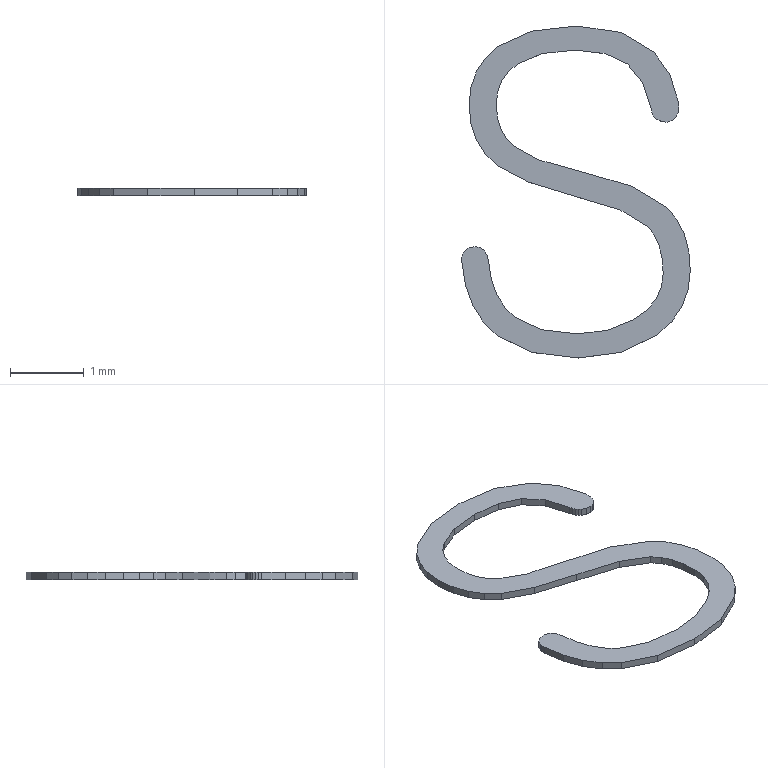Part | STEP file | PART234.stp | 1 solid | 96 faces | box 3.09 x 4.487 x 0.1 mm | volume 0.3955 mm3 | plane 96